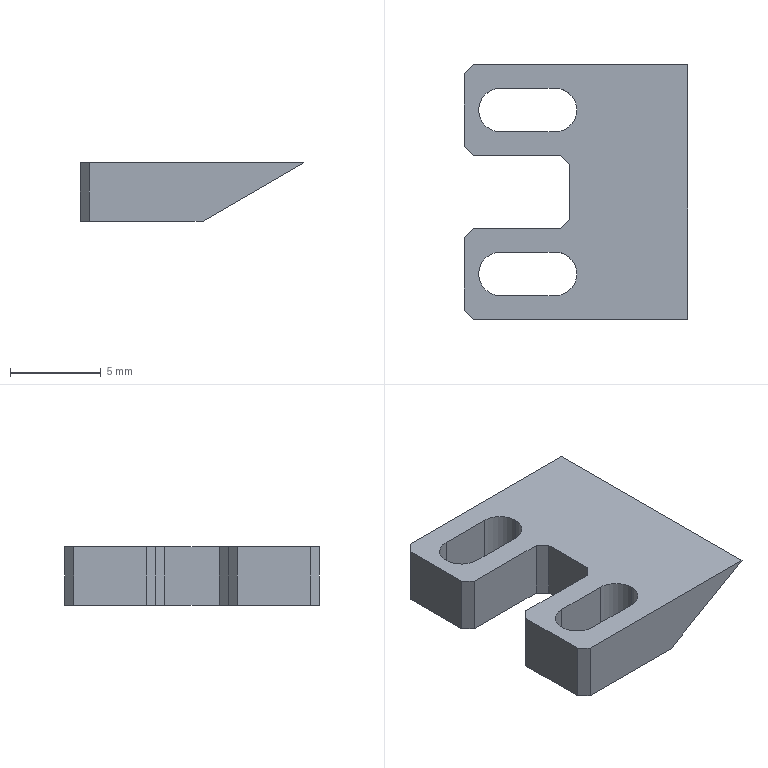CAM job | NX | 3-axis milling | part box 12.3 x 14 x 3.2 mm | stock box 16.3 x 18 x 4.2 mm
Tools:
number,name,description,diameter,corner_radius,flute_length,length,flutes
9,D10JING,Milling Tool-5 Parameters,10.0,0.0,50.0,75.0,2
6,D6,Milling Tool-5 Parameters,6.0,0.0,50.0,75.0,2
2,D2,Milling Tool-5 Parameters,2.0,0.0,50.0,75.0,2
7,D6A45,Milling Tool-5 Parameters,6.0,0.0,50.0,75.0,2
5,D2R0.5,Milling Tool-5 Parameters,2.0,0.5,50.0,75.0,2
Operations:
program,operation,operation_type,tool,method,geometry_group,spindle_rpm,surface_speed,feed_per_tooth,feed_cut,feed_plunge,cut_length_mm,path_length_mm,cut_time_min,machine_time_min
1,FLOOR_WALL,VolumeBased25DMillingOperation,D10JING,METHOD,A,9500.0,298.0,0.0658,1250.0,100.0,136.297,190.297,0.109,0.1144
1,ZLEVEL_PROFILE,ZLevelMilling,D6,METHOD,A,9500.0,298.0,0.1316,2500.0,1000.0,533.764,593.814,0.2357,0.2417
1,ZLEVEL_PROFILE_COPY_1,ZLevelMilling,D2,METHOD,A,9500.0,298.0,0.1316,2500.0,1000.0,1361.394,1422.444,0.5577,0.5638
1,ZLEVEL_PROFILE_COPY_1_COPY,ZLevelMilling,D2,METHOD,A,9500.0,298.0,0.1316,2500.0,1000.0,375.338,506.863,0.1764,0.1896
1,PLANAR_MILL_COPY_1_COPY,PlanarMilling,D6A45,METHOD,A,9500.0,179.0,0.0658,1250.0,100.0,76.542,282.346,0.0612,0.0818
1,ZLEVEL_PROFILE_1,ZLevelMilling,D2R0.5,METHOD,A,9500.0,89.0,0.1316,2500.0,1000.0,1315.309,1372.829,0.5282,0.534
1,刀补6,ZLevelMilling,D2,METHOD,A,9500.0,298.0,0.0632,1200.0,1000.0,76.68,138.78,0.0646,0.0708